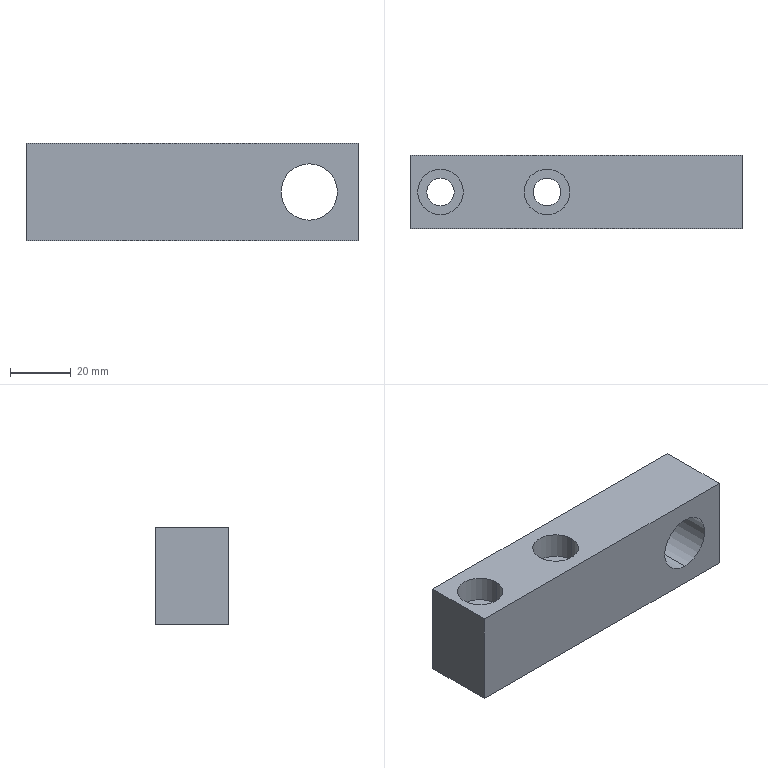Part | STEP file | PN_0006 (buffer fixed block) | 1 solid | 24 faces | box 109 x 24 x 32 mm | volume 69208 mm3 | cylinder 14 | plane 10 | commonest cylinder face diameters 15 x8 9 x4 18.5 x2